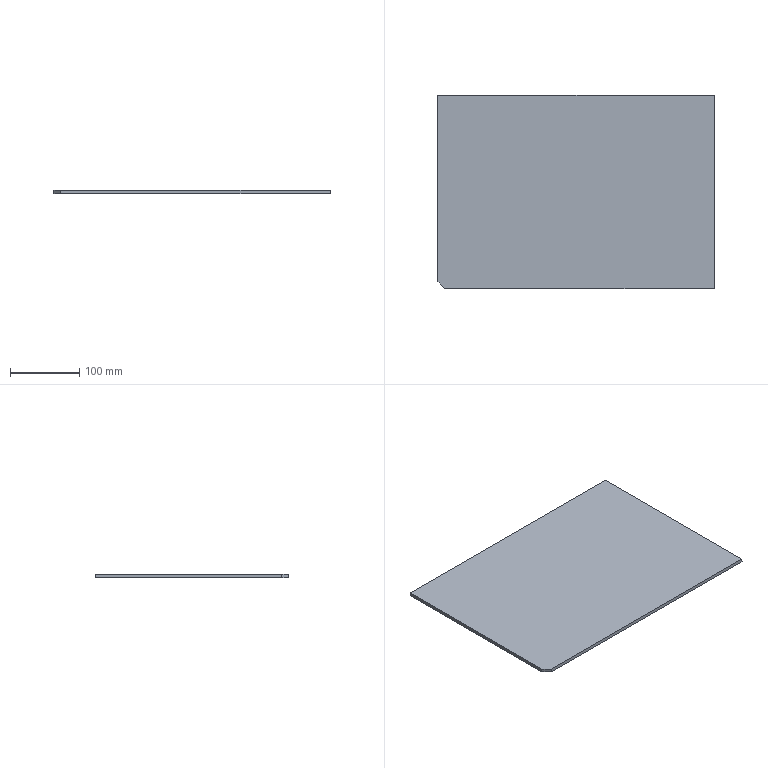Part | SolidWorks | features Chamfer 1, FlatPattern 1, ICE 1, LPattern 1, SMBaseFlange 1, SheetMetal 1 | 1 solid | 7 faces | box 400 x 280 x 5 mm | volume 559750 mm3 | plane 7
STEP:
#1=CARTESIAN_POINT('',(200.,-140.,0.));
#2=VERTEX_POINT('',#1);
#3=CARTESIAN_POINT('',(200.,140.,0.));
#4=VERTEX_POINT('',#3);
#5=CARTESIAN_POINT('',(200.,-140.,0.));
#6=DIRECTION('',(0.,1.,0.));
#7=VECTOR('',#6,1000.);
#8=LINE('',#5,#7);
#9=EDGE_CURVE('',#2,#4,#8,.T.);
#10=ORIENTED_EDGE('',*,*,#9,.F.);
#11=CARTESIAN_POINT('',(200.,-140.,-5.));
#12=VERTEX_POINT('',#11);
#13=CARTESIAN_POINT('',(200.,-140.,-5.));
#14=DIRECTION('',(0.,0.,1.));
#15=VECTOR('',#14,1000.);
#16=LINE('',#13,#15);
#17=EDGE_CURVE('',#12,#2,#16,.T.);
#18=ORIENTED_EDGE('',*,*,#17,.F.);
#19=CARTESIAN_POINT('',(200.,140.,-5.));
#20=VERTEX_POINT('',#19);
#21=CARTESIAN_POINT('',(200.,-140.,-5.));
#22=DIRECTION('',(0.,1.,0.));
#23=VECTOR('',#22,1000.);
#24=LINE('',#21,#23);
#25=EDGE_CURVE('',#12,#20,#24,.T.);
#26=ORIENTED_EDGE('',*,*,#25,.T.);
#27=CARTESIAN_POINT('',(200.,140.,-5.));
#28=DIRECTION('',(0.,0.,1.));
#29=VECTOR('',#28,1000.);
#30=LINE('',#27,#29);
#31=EDGE_CURVE('',#20,#4,#30,.T.);
#32=ORIENTED_EDGE('',*,*,#31,.T.);
#33=EDGE_LOOP('',(#10,#18,#26,#32));
#34=FACE_OUTER_BOUND('',#33,.T.);
#35=CARTESIAN_POINT('',(200.,-140.,-5.));
#36=DIRECTION('',(1.,0.,0.));
#37=DIRECTION('',(0.,0.,-1.));
#38=AXIS2_PLACEMENT_3D('',#35,#36,#37);
#39=PLANE('',#38);
#40=ADVANCED_FACE('',(#34),#39,.T.);
#41=CARTESIAN_POINT('',(-190.,-140.,0.));
#42=VERTEX_POINT('',#41);
#43=CARTESIAN_POINT('',(-200.,-140.,0.));
#44=DIRECTION('',(1.,0.,0.));
#45=VECTOR('',#44,1000.);
#46=LINE('',#43,#45);
#47=EDGE_CURVE('',#42,#2,#46,.T.);
#48=ORIENTED_EDGE('',*,*,#47,.F.);
#49=CARTESIAN_POINT('',(-190.,-140.,-5.));
#50=VERTEX_POINT('',#49);
#51=CARTESIAN_POINT('',(-190.,-140.,-5.));
#52=DIRECTION('',(0.,0.,-1.));
#53=VECTOR('',#52,1000.);
#54=LINE('',#51,#53);
#55=EDGE_CURVE('',#42,#50,#54,.T.);
#56=ORIENTED_EDGE('',*,*,#55,.T.);
#57=CARTESIAN_POINT('',(-200.,-140.,-5.));
#58=DIRECTION('',(1.,0.,0.));
#59=VECTOR('',#58,1000.);
#60=LINE('',#57,#59);
#61=EDGE_CURVE('',#50,#12,#60,.T.);
#62=ORIENTED_EDGE('',*,*,#61,.T.);
#63=ORIENTED_EDGE('',*,*,#17,.T.);
#64=EDGE_LOOP('',(#48,#56,#62,#63));
#65=FACE_OUTER_BOUND('',#64,.T.);
#66=CARTESIAN_POINT('',(-200.,-140.,-5.));
#67=DIRECTION('',(0.,-1.,0.));
#68=DIRECTION('',(0.,0.,-1.));
#69=AXIS2_PLACEMENT_3D('',#66,#67,#68);
#70=PLANE('',#69);
#71=ADVANCED_FACE('',(#65),#70,.T.);
#72=CARTESIAN_POINT('',(-200.,140.,-5.));
#73=VERTEX_POINT('',#72);
#74=CARTESIAN_POINT('',(-200.,-130.,-5.));
#75=VERTEX_POINT('',#74);
#76=CARTESIAN_POINT('',(-200.,-140.,-5.));
#77=DIRECTION('',(0.,-1.,0.));
#78=VECTOR('',#77,1000.);
#79=LINE('',#76,#78);
#80=EDGE_CURVE('',#73,#75,#79,.T.);
#81=ORIENTED_EDGE('',*,*,#80,.T.);
#82=CARTESIAN_POINT('',(-200.,-130.,0.));
#83=VERTEX_POINT('',#82);
#84=CARTESIAN_POINT('',(-200.,-130.,-5.));
#85=DIRECTION('',(0.,0.,1.));
#86=VECTOR('',#85,1000.);
#87=LINE('',#84,#86);
#88=EDGE_CURVE('',#75,#83,#87,.T.);
#89=ORIENTED_EDGE('',*,*,#88,.T.);
#90=CARTESIAN_POINT('',(-200.,140.,0.));
#91=VERTEX_POINT('',#90);
#92=CARTESIAN_POINT('',(-200.,-140.,0.));
#93=DIRECTION('',(0.,-1.,0.));
#94=VECTOR('',#93,1000.);
#95=LINE('',#92,#94);
#96=EDGE_CURVE('',#91,#83,#95,.T.);
#97=ORIENTED_EDGE('',*,*,#96,.F.);
#98=CARTESIAN_POINT('',(-200.,140.,-5.));
#99=DIRECTION('',(0.,0.,1.));
#100=VECTOR('',#99,1000.);
#101=LINE('',#98,#100);
#102=EDGE_CURVE('',#73,#91,#101,.T.);
#103=ORIENTED_EDGE('',*,*,#102,.F.);
#104=EDGE_LOOP('',(#81,#89,#97,#103));
#105=FACE_OUTER_BOUND('',#104,.T.);
#106=CARTESIAN_POINT('',(-200.,-140.,-5.));
#107=DIRECTION('',(-1.,0.,0.));
#108=DIRECTION('',(0.,0.,1.));
#109=AXIS2_PLACEMENT_3D('',#106,#107,#108);
#110=PLANE('',#109);
#111=ADVANCED_FACE('',(#105),#110,.T.);
#112=CARTESIAN_POINT('',(-200.,140.,0.));
#113=DIRECTION('',(-1.,0.,0.));
#114=VECTOR('',#113,1000.);
#115=LINE('',#112,#114);
#116=EDGE_CURVE('',#4,#91,#115,.T.);
#117=ORIENTED_EDGE('',*,*,#116,.F.);
#118=ORIENTED_EDGE('',*,*,#31,.F.);
#119=CARTESIAN_POINT('',(-200.,140.,-5.));
#120=DIRECTION('',(-1.,0.,0.));
#121=VECTOR('',#120,1000.);
#122=LINE('',#119,#121);
#123=EDGE_CURVE('',#20,#73,#122,.T.);
#124=ORIENTED_EDGE('',*,*,#123,.T.);
#125=ORIENTED_EDGE('',*,*,#102,.T.);
#126=EDGE_LOOP('',(#117,#118,#124,#125));
#127=FACE_OUTER_BOUND('',#126,.T.);
#128=CARTESIAN_POINT('',(-200.,140.,-5.));
#129=DIRECTION('',(0.,1.,0.));
#130=DIRECTION('',(0.,0.,1.));
#131=AXIS2_PLACEMENT_3D('',#128,#129,#130);
#132=PLANE('',#131);
#133=ADVANCED_FACE('',(#127),#132,.T.);
#134=ORIENTED_EDGE('',*,*,#61,.F.);
#135=CARTESIAN_POINT('',(-165.,-165.,-5.));
#136=DIRECTION('',(-0.7071,0.7071,0.));
#137=VECTOR('',#136,1000.);
#138=LINE('',#135,#137);
#139=EDGE_CURVE('',#50,#75,#138,.T.);
#140=ORIENTED_EDGE('',*,*,#139,.T.);
#141=ORIENTED_EDGE('',*,*,#80,.F.);
#142=ORIENTED_EDGE('',*,*,#123,.F.);
#143=ORIENTED_EDGE('',*,*,#25,.F.);
#144=EDGE_LOOP('',(#134,#140,#141,#142,#143));
#145=FACE_OUTER_BOUND('',#144,.T.);
#146=CARTESIAN_POINT('',(0.,0.,-5.));
#147=DIRECTION('',(0.,0.,-1.));
#148=DIRECTION('',(-1.,0.,0.));
#149=AXIS2_PLACEMENT_3D('',#146,#147,#148);
#150=PLANE('',#149);
#151=ADVANCED_FACE('',(#145),#150,.T.);
#152=ORIENTED_EDGE('',*,*,#96,.T.);
#153=CARTESIAN_POINT('',(-200.,-130.,0.));
#154=DIRECTION('',(0.7071,-0.7071,0.));
#155=VECTOR('',#154,1000.);
#156=LINE('',#153,#155);
#157=EDGE_CURVE('',#83,#42,#156,.T.);
#158=ORIENTED_EDGE('',*,*,#157,.T.);
#159=ORIENTED_EDGE('',*,*,#47,.T.);
#160=ORIENTED_EDGE('',*,*,#9,.T.);
#161=ORIENTED_EDGE('',*,*,#116,.T.);
#162=EDGE_LOOP('',(#152,#158,#159,#160,#161));
#163=FACE_OUTER_BOUND('',#162,.T.);
#164=CARTESIAN_POINT('',(0.,0.,0.));
#165=DIRECTION('',(0.,0.,-1.));
#166=DIRECTION('',(-1.,0.,0.));
#167=AXIS2_PLACEMENT_3D('',#164,#165,#166);
#168=PLANE('',#167);
#169=ADVANCED_FACE('',(#163),#168,.F.);
#170=ORIENTED_EDGE('',*,*,#139,.F.);
#171=ORIENTED_EDGE('',*,*,#55,.F.);
#172=ORIENTED_EDGE('',*,*,#157,.F.);
#173=ORIENTED_EDGE('',*,*,#88,.F.);
#174=EDGE_LOOP('',(#170,#171,#172,#173));
#175=FACE_OUTER_BOUND('',#174,.T.);
#176=CARTESIAN_POINT('',(-200.,-130.,-5.));
#177=DIRECTION('',(0.7071,0.7071,0.));
#178=DIRECTION('',(0.,0.,1.));
#179=AXIS2_PLACEMENT_3D('',#176,#177,#178);
#180=PLANE('',#179);
#181=ADVANCED_FACE('',(#175),#180,.F.);
#182=CLOSED_SHELL('',(#40,#71,#111,#133,#151,#169,#181));
#183=MANIFOLD_SOLID_BREP('',#182);
#184=CARTESIAN_POINT('',(0.,0.,0.));
#185=DIRECTION('',(0.,0.,1.));
#186=DIRECTION('',(1.,0.,0.));
#187=AXIS2_PLACEMENT_3D('',#184,#185,#186);
#188=(LENGTH_UNIT()NAMED_UNIT(*)SI_UNIT(.MILLI.,.METRE.));
#189=UNCERTAINTY_MEASURE_WITH_UNIT(LENGTH_MEASURE(0.00001),#188,'','');
#190=(NAMED_UNIT(*)PLANE_ANGLE_UNIT()SI_UNIT($,.RADIAN.));
#191=(NAMED_UNIT(*)SI_UNIT($,.STERADIAN.)SOLID_ANGLE_UNIT());
#192=(GEOMETRIC_REPRESENTATION_CONTEXT(3)GLOBAL_UNCERTAINTY_ASSIGNED_CONTEXT((#189))GLOBAL_UNIT_ASSIGNED_CONTEXT((#188,#190,#191))REPRESENTATION_CONTEXT('',''));
#193=ADVANCED_BREP_SHAPE_REPRESENTATION('',(#183,#187),#192);